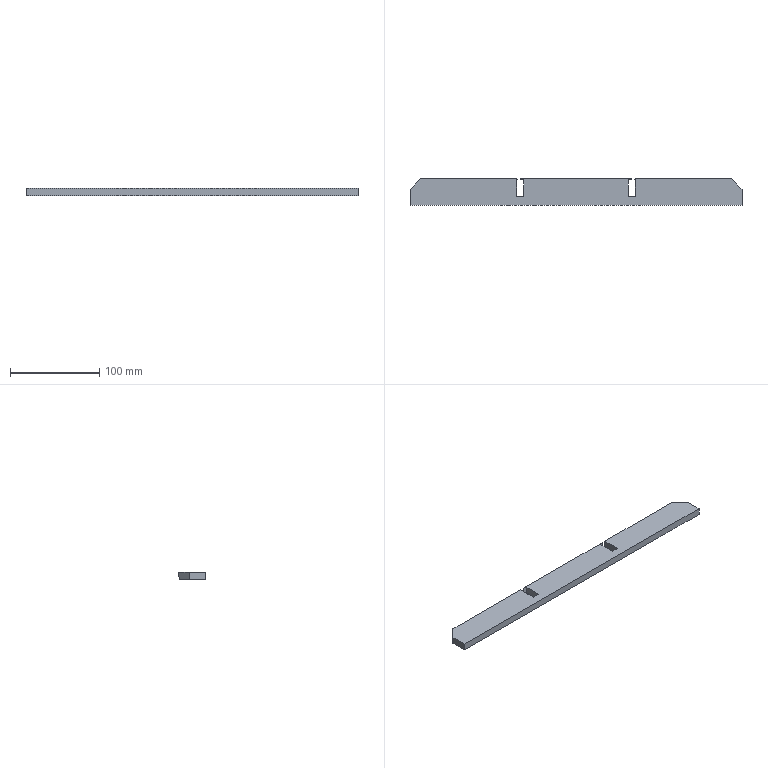Part | SolidWorks | features BaseBody 1 | 1 solid | 18 faces | box 373 x 30 x 8 mm | volume 84961 mm3 | plane 18
STEP:
#1=CARTESIAN_POINT('',(62.311,14.398,0.));
#2=VERTEX_POINT('',#1);
#3=CARTESIAN_POINT('',(62.597,15.,8.));
#4=VERTEX_POINT('',#3);
#5=CARTESIAN_POINT('',(62.311,14.398,0.));
#6=DIRECTION('',(0.0356,0.07493,0.9966));
#7=VECTOR('',#6,1000.);
#8=LINE('',#5,#7);
#9=EDGE_CURVE('',#2,#4,#8,.T.);
#10=ORIENTED_EDGE('',*,*,#9,.F.);
#11=CARTESIAN_POINT('',(-62.311,14.398,0.));
#12=VERTEX_POINT('',#11);
#13=CARTESIAN_POINT('',(0.,14.398,0.));
#14=DIRECTION('',(1.,0.,0.));
#15=VECTOR('',#14,1000.);
#16=LINE('',#13,#15);
#17=EDGE_CURVE('',#12,#2,#16,.T.);
#18=ORIENTED_EDGE('',*,*,#17,.F.);
#19=CARTESIAN_POINT('',(-62.597,15.,8.));
#20=VERTEX_POINT('',#19);
#21=CARTESIAN_POINT('',(-62.597,15.,8.));
#22=DIRECTION('',(0.0356,-0.07493,-0.9966));
#23=VECTOR('',#22,1000.);
#24=LINE('',#21,#23);
#25=EDGE_CURVE('',#20,#12,#24,.T.);
#26=ORIENTED_EDGE('',*,*,#25,.F.);
#27=CARTESIAN_POINT('',(0.,15.,8.));
#28=DIRECTION('',(-1.,0.,0.));
#29=VECTOR('',#28,1000.);
#30=LINE('',#27,#29);
#31=EDGE_CURVE('',#4,#20,#30,.T.);
#32=ORIENTED_EDGE('',*,*,#31,.F.);
#33=EDGE_LOOP('',(#10,#18,#26,#32));
#34=FACE_OUTER_BOUND('',#33,.T.);
#35=CARTESIAN_POINT('',(-63.348,15.,8.));
#36=DIRECTION('',(0.,-0.9972,0.07498));
#37=DIRECTION('',(0.,-0.07498,-0.9972));
#38=AXIS2_PLACEMENT_3D('',#35,#36,#37);
#39=PLANE('',#38);
#40=ADVANCED_FACE('',(#34),#39,.F.);
#41=CARTESIAN_POINT('',(58.61,14.882,8.));
#42=VERTEX_POINT('',#41);
#43=CARTESIAN_POINT('',(62.597,15.,8.));
#44=DIRECTION('',(-0.9996,-0.02956,0.));
#45=VECTOR('',#44,1000.);
#46=LINE('',#43,#45);
#47=EDGE_CURVE('',#4,#42,#46,.T.);
#48=ORIENTED_EDGE('',*,*,#47,.F.);
#49=ORIENTED_EDGE('',*,*,#31,.T.);
#50=CARTESIAN_POINT('',(-58.61,14.882,8.));
#51=VERTEX_POINT('',#50);
#52=CARTESIAN_POINT('',(-58.61,14.882,8.));
#53=DIRECTION('',(-0.9996,0.02956,0.));
#54=VECTOR('',#53,1000.);
#55=LINE('',#52,#54);
#56=EDGE_CURVE('',#51,#20,#55,.T.);
#57=ORIENTED_EDGE('',*,*,#56,.F.);
#58=CARTESIAN_POINT('',(-59.134,-5.166,8.));
#59=VERTEX_POINT('',#58);
#60=CARTESIAN_POINT('',(-59.134,-5.166,8.));
#61=DIRECTION('',(0.02613,0.9997,0.));
#62=VECTOR('',#61,1000.);
#63=LINE('',#60,#62);
#64=EDGE_CURVE('',#59,#51,#63,.T.);
#65=ORIENTED_EDGE('',*,*,#64,.F.);
#66=CARTESIAN_POINT('',(-67.139,-4.929,8.));
#67=VERTEX_POINT('',#66);
#68=CARTESIAN_POINT('',(-67.139,-4.929,8.));
#69=DIRECTION('',(0.9996,-0.02956,0.));
#70=VECTOR('',#69,1000.);
#71=LINE('',#68,#70);
#72=EDGE_CURVE('',#67,#59,#71,.T.);
#73=ORIENTED_EDGE('',*,*,#72,.F.);
#74=CARTESIAN_POINT('',(-66.618,15.,8.));
#75=VERTEX_POINT('',#74);
#76=CARTESIAN_POINT('',(-66.618,15.,8.));
#77=DIRECTION('',(-0.02613,-0.9997,0.));
#78=VECTOR('',#77,1000.);
#79=LINE('',#76,#78);
#80=EDGE_CURVE('',#75,#67,#79,.T.);
#81=ORIENTED_EDGE('',*,*,#80,.F.);
#82=CARTESIAN_POINT('',(-174.5,15.,8.));
#83=VERTEX_POINT('',#82);
#84=CARTESIAN_POINT('',(0.,15.,8.));
#85=DIRECTION('',(1.,0.,0.));
#86=VECTOR('',#85,1000.);
#87=LINE('',#84,#86);
#88=EDGE_CURVE('',#83,#75,#87,.T.);
#89=ORIENTED_EDGE('',*,*,#88,.F.);
#90=CARTESIAN_POINT('',(-186.5,3.,8.));
#91=VERTEX_POINT('',#90);
#92=CARTESIAN_POINT('',(-186.5,3.,8.));
#93=DIRECTION('',(0.7071,0.7071,0.));
#94=VECTOR('',#93,1000.);
#95=LINE('',#92,#94);
#96=EDGE_CURVE('',#91,#83,#95,.T.);
#97=ORIENTED_EDGE('',*,*,#96,.F.);
#98=CARTESIAN_POINT('',(-186.5,-15.,8.));
#99=VERTEX_POINT('',#98);
#100=CARTESIAN_POINT('',(-186.5,0.,8.));
#101=DIRECTION('',(0.,1.,0.));
#102=VECTOR('',#101,1000.);
#103=LINE('',#100,#102);
#104=EDGE_CURVE('',#99,#91,#103,.T.);
#105=ORIENTED_EDGE('',*,*,#104,.F.);
#106=CARTESIAN_POINT('',(186.5,-15.,8.));
#107=VERTEX_POINT('',#106);
#108=CARTESIAN_POINT('',(0.,-15.,8.));
#109=DIRECTION('',(-1.,0.,0.));
#110=VECTOR('',#109,1000.);
#111=LINE('',#108,#110);
#112=EDGE_CURVE('',#107,#99,#111,.T.);
#113=ORIENTED_EDGE('',*,*,#112,.F.);
#114=CARTESIAN_POINT('',(186.5,3.,8.));
#115=VERTEX_POINT('',#114);
#116=CARTESIAN_POINT('',(186.5,0.,8.));
#117=DIRECTION('',(0.,-1.,0.));
#118=VECTOR('',#117,1000.);
#119=LINE('',#116,#118);
#120=EDGE_CURVE('',#115,#107,#119,.T.);
#121=ORIENTED_EDGE('',*,*,#120,.F.);
#122=CARTESIAN_POINT('',(174.5,15.,8.));
#123=VERTEX_POINT('',#122);
#124=CARTESIAN_POINT('',(174.428,15.072,8.));
#125=DIRECTION('',(0.7071,-0.7071,0.));
#126=VECTOR('',#125,1000.);
#127=LINE('',#124,#126);
#128=EDGE_CURVE('',#123,#115,#127,.T.);
#129=ORIENTED_EDGE('',*,*,#128,.F.);
#130=CARTESIAN_POINT('',(66.618,15.,8.));
#131=VERTEX_POINT('',#130);
#132=CARTESIAN_POINT('',(0.,15.,8.));
#133=DIRECTION('',(1.,0.,0.));
#134=VECTOR('',#133,1000.);
#135=LINE('',#132,#134);
#136=EDGE_CURVE('',#131,#123,#135,.T.);
#137=ORIENTED_EDGE('',*,*,#136,.F.);
#138=CARTESIAN_POINT('',(67.139,-4.929,8.));
#139=VERTEX_POINT('',#138);
#140=CARTESIAN_POINT('',(67.139,-4.929,8.));
#141=DIRECTION('',(-0.02613,0.9997,0.));
#142=VECTOR('',#141,1000.);
#143=LINE('',#140,#142);
#144=EDGE_CURVE('',#139,#131,#143,.T.);
#145=ORIENTED_EDGE('',*,*,#144,.F.);
#146=CARTESIAN_POINT('',(59.134,-5.166,8.));
#147=VERTEX_POINT('',#146);
#148=CARTESIAN_POINT('',(59.134,-5.166,8.));
#149=DIRECTION('',(0.9996,0.02956,0.));
#150=VECTOR('',#149,1000.);
#151=LINE('',#148,#150);
#152=EDGE_CURVE('',#147,#139,#151,.T.);
#153=ORIENTED_EDGE('',*,*,#152,.F.);
#154=CARTESIAN_POINT('',(58.61,14.882,8.));
#155=DIRECTION('',(0.02613,-0.9997,0.));
#156=VECTOR('',#155,1000.);
#157=LINE('',#154,#156);
#158=EDGE_CURVE('',#42,#147,#157,.T.);
#159=ORIENTED_EDGE('',*,*,#158,.F.);
#160=EDGE_LOOP('',(#48,#49,#57,#65,#73,#81,#89,#97,#105,#113,#121,#129,#137,#145,#153,#159));
#161=FACE_OUTER_BOUND('',#160,.T.);
#162=CARTESIAN_POINT('',(186.5,-15.,8.));
#163=DIRECTION('',(0.,0.,-1.));
#164=DIRECTION('',(-1.,0.,0.));
#165=AXIS2_PLACEMENT_3D('',#162,#163,#164);
#166=PLANE('',#165);
#167=ADVANCED_FACE('',(#161),#166,.F.);
#168=CARTESIAN_POINT('',(58.255,14.279,0.));
#169=VERTEX_POINT('',#168);
#170=CARTESIAN_POINT('',(62.311,14.398,0.));
#171=DIRECTION('',(-0.9996,-0.02956,0.));
#172=VECTOR('',#171,1000.);
#173=LINE('',#170,#172);
#174=EDGE_CURVE('',#2,#169,#173,.T.);
#175=ORIENTED_EDGE('',*,*,#174,.F.);
#176=ORIENTED_EDGE('',*,*,#9,.T.);
#177=ORIENTED_EDGE('',*,*,#47,.T.);
#178=CARTESIAN_POINT('',(58.255,14.279,0.000000002));
#179=DIRECTION('',(0.04418,0.07516,0.9962));
#180=VECTOR('',#179,1000.);
#181=LINE('',#178,#180);
#182=EDGE_CURVE('',#169,#42,#181,.T.);
#183=ORIENTED_EDGE('',*,*,#182,.F.);
#184=EDGE_LOOP('',(#175,#176,#177,#183));
#185=FACE_OUTER_BOUND('',#184,.T.);
#186=CARTESIAN_POINT('',(58.229,14.274,-0.048));
#187=DIRECTION('',(-0.02948,0.9968,-0.0739));
#188=DIRECTION('',(0.,0.07393,0.9973));
#189=AXIS2_PLACEMENT_3D('',#186,#187,#188);
#190=PLANE('',#189);
#191=ADVANCED_FACE('',(#185),#190,.F.);
#192=CARTESIAN_POINT('',(-58.255,14.279,0.));
#193=VERTEX_POINT('',#192);
#194=CARTESIAN_POINT('',(-58.255,14.279,0.));
#195=DIRECTION('',(-0.9996,0.02956,0.));
#196=VECTOR('',#195,1000.);
#197=LINE('',#194,#196);
#198=EDGE_CURVE('',#193,#12,#197,.T.);
#199=ORIENTED_EDGE('',*,*,#198,.T.);
#200=ORIENTED_EDGE('',*,*,#17,.T.);
#201=ORIENTED_EDGE('',*,*,#174,.T.);
#202=CARTESIAN_POINT('',(58.779,-5.77,0.));
#203=VERTEX_POINT('',#202);
#204=CARTESIAN_POINT('',(58.255,14.279,0.));
#205=DIRECTION('',(0.02613,-0.9997,0.));
#206=VECTOR('',#205,1000.);
#207=LINE('',#204,#206);
#208=EDGE_CURVE('',#169,#203,#207,.T.);
#209=ORIENTED_EDGE('',*,*,#208,.T.);
#210=CARTESIAN_POINT('',(66.784,-5.533,0.));
#211=VERTEX_POINT('',#210);
#212=CARTESIAN_POINT('',(58.779,-5.77,0.));
#213=DIRECTION('',(0.9996,0.02956,0.));
#214=VECTOR('',#213,1000.);
#215=LINE('',#212,#214);
#216=EDGE_CURVE('',#203,#211,#215,.T.);
#217=ORIENTED_EDGE('',*,*,#216,.T.);
#218=CARTESIAN_POINT('',(66.263,14.398,0.));
#219=VERTEX_POINT('',#218);
#220=CARTESIAN_POINT('',(66.784,-5.533,0.));
#221=DIRECTION('',(-0.02613,0.9997,0.));
#222=VECTOR('',#221,1000.);
#223=LINE('',#220,#222);
#224=EDGE_CURVE('',#211,#219,#223,.T.);
#225=ORIENTED_EDGE('',*,*,#224,.T.);
#226=CARTESIAN_POINT('',(175.102,14.398,0.));
#227=VERTEX_POINT('',#226);
#228=CARTESIAN_POINT('',(0.,14.398,0.));
#229=DIRECTION('',(1.,0.,0.));
#230=VECTOR('',#229,1000.);
#231=LINE('',#228,#230);
#232=EDGE_CURVE('',#219,#227,#231,.T.);
#233=ORIENTED_EDGE('',*,*,#232,.T.);
#234=CARTESIAN_POINT('',(186.5,3.,0.));
#235=VERTEX_POINT('',#234);
#236=CARTESIAN_POINT('',(175.102,14.398,0.));
#237=DIRECTION('',(0.7071,-0.7071,0.));
#238=VECTOR('',#237,1000.);
#239=LINE('',#236,#238);
#240=EDGE_CURVE('',#227,#235,#239,.T.);
#241=ORIENTED_EDGE('',*,*,#240,.T.);
#242=CARTESIAN_POINT('',(186.5,-15.,0.));
#243=VERTEX_POINT('',#242);
#244=CARTESIAN_POINT('',(186.5,-0.3008,0.));
#245=DIRECTION('',(0.,-1.,0.));
#246=VECTOR('',#245,1000.);
#247=LINE('',#244,#246);
#248=EDGE_CURVE('',#235,#243,#247,.T.);
#249=ORIENTED_EDGE('',*,*,#248,.T.);
#250=CARTESIAN_POINT('',(-186.5,-15.,0.));
#251=VERTEX_POINT('',#250);
#252=CARTESIAN_POINT('',(0.,-15.,0.));
#253=DIRECTION('',(-1.,0.,0.));
#254=VECTOR('',#253,1000.);
#255=LINE('',#252,#254);
#256=EDGE_CURVE('',#243,#251,#255,.T.);
#257=ORIENTED_EDGE('',*,*,#256,.T.);
#258=CARTESIAN_POINT('',(-186.5,3.,0.));
#259=VERTEX_POINT('',#258);
#260=CARTESIAN_POINT('',(-186.5,-0.3008,0.));
#261=DIRECTION('',(0.,1.,0.));
#262=VECTOR('',#261,1000.);
#263=LINE('',#260,#262);
#264=EDGE_CURVE('',#251,#259,#263,.T.);
#265=ORIENTED_EDGE('',*,*,#264,.T.);
#266=CARTESIAN_POINT('',(-175.102,14.398,0.));
#267=VERTEX_POINT('',#266);
#268=CARTESIAN_POINT('',(-186.5,3.,0.));
#269=DIRECTION('',(0.7071,0.7071,0.));
#270=VECTOR('',#269,1000.);
#271=LINE('',#268,#270);
#272=EDGE_CURVE('',#259,#267,#271,.T.);
#273=ORIENTED_EDGE('',*,*,#272,.T.);
#274=CARTESIAN_POINT('',(-66.263,14.398,0.));
#275=VERTEX_POINT('',#274);
#276=CARTESIAN_POINT('',(0.,14.398,0.));
#277=DIRECTION('',(1.,0.,0.));
#278=VECTOR('',#277,1000.);
#279=LINE('',#276,#278);
#280=EDGE_CURVE('',#267,#275,#279,.T.);
#281=ORIENTED_EDGE('',*,*,#280,.T.);
#282=CARTESIAN_POINT('',(-66.784,-5.533,0.));
#283=VERTEX_POINT('',#282);
#284=CARTESIAN_POINT('',(-66.263,14.398,0.));
#285=DIRECTION('',(-0.02613,-0.9997,0.));
#286=VECTOR('',#285,1000.);
#287=LINE('',#284,#286);
#288=EDGE_CURVE('',#275,#283,#287,.T.);
#289=ORIENTED_EDGE('',*,*,#288,.T.);
#290=CARTESIAN_POINT('',(-58.779,-5.77,0.));
#291=VERTEX_POINT('',#290);
#292=CARTESIAN_POINT('',(-66.784,-5.533,0.));
#293=DIRECTION('',(0.9996,-0.02956,0.));
#294=VECTOR('',#293,1000.);
#295=LINE('',#292,#294);
#296=EDGE_CURVE('',#283,#291,#295,.T.);
#297=ORIENTED_EDGE('',*,*,#296,.T.);
#298=CARTESIAN_POINT('',(-58.779,-5.77,0.));
#299=DIRECTION('',(0.02613,0.9997,0.));
#300=VECTOR('',#299,1000.);
#301=LINE('',#298,#300);
#302=EDGE_CURVE('',#291,#193,#301,.T.);
#303=ORIENTED_EDGE('',*,*,#302,.T.);
#304=EDGE_LOOP('',(#199,#200,#201,#209,#217,#225,#233,#241,#249,#257,#265,#273,#281,#289,#297,#303));
#305=FACE_OUTER_BOUND('',#304,.T.);
#306=CARTESIAN_POINT('',(186.5,-15.,0.));
#307=DIRECTION('',(0.,0.,-1.));
#308=DIRECTION('',(-1.,0.,0.));
#309=AXIS2_PLACEMENT_3D('',#306,#307,#308);
#310=PLANE('',#309);
#311=ADVANCED_FACE('',(#305),#310,.T.);
#312=ORIENTED_EDGE('',*,*,#198,.F.);
#313=CARTESIAN_POINT('',(-58.61,14.882,8.));
#314=DIRECTION('',(0.04418,-0.07516,-0.9962));
#315=VECTOR('',#314,1000.);
#316=LINE('',#313,#315);
#317=EDGE_CURVE('',#51,#193,#316,.T.);
#318=ORIENTED_EDGE('',*,*,#317,.F.);
#319=ORIENTED_EDGE('',*,*,#56,.T.);
#320=ORIENTED_EDGE('',*,*,#25,.T.);
#321=EDGE_LOOP('',(#312,#318,#319,#320));
#322=FACE_OUTER_BOUND('',#321,.T.);
#323=CARTESIAN_POINT('',(-62.623,14.403,-0.05758));
#324=DIRECTION('',(0.02948,0.9968,-0.0739));
#325=DIRECTION('',(0.,0.07393,0.9973));
#326=AXIS2_PLACEMENT_3D('',#323,#324,#325);
#327=PLANE('',#326);
#328=ADVANCED_FACE('',(#322),#327,.F.);
#329=ORIENTED_EDGE('',*,*,#208,.F.);
#330=ORIENTED_EDGE('',*,*,#182,.T.);
#331=ORIENTED_EDGE('',*,*,#158,.T.);
#332=CARTESIAN_POINT('',(58.779,-5.77,0.000000003));
#333=DIRECTION('',(0.04418,0.07516,0.9962));
#334=VECTOR('',#333,1000.);
#335=LINE('',#332,#334);
#336=EDGE_CURVE('',#203,#147,#335,.T.);
#337=ORIENTED_EDGE('',*,*,#336,.F.);
#338=EDGE_LOOP('',(#329,#330,#331,#337));
#339=FACE_OUTER_BOUND('',#338,.T.);
#340=CARTESIAN_POINT('',(58.779,-5.893,-0.07251));
#341=DIRECTION('',(-0.9986,-0.0261,0.04626));
#342=DIRECTION('',(0.04627,0.,0.9989));
#343=AXIS2_PLACEMENT_3D('',#340,#341,#342);
#344=PLANE('',#343);
#345=ADVANCED_FACE('',(#339),#344,.F.);
#346=ORIENTED_EDGE('',*,*,#302,.F.);
#347=CARTESIAN_POINT('',(-59.134,-5.166,8.));
#348=DIRECTION('',(0.04418,-0.07516,-0.9962));
#349=VECTOR('',#348,1000.);
#350=LINE('',#347,#349);
#351=EDGE_CURVE('',#59,#291,#350,.T.);
#352=ORIENTED_EDGE('',*,*,#351,.F.);
#353=ORIENTED_EDGE('',*,*,#64,.T.);
#354=ORIENTED_EDGE('',*,*,#317,.T.);
#355=EDGE_LOOP('',(#346,#352,#353,#354));
#356=FACE_OUTER_BOUND('',#355,.T.);
#357=CARTESIAN_POINT('',(-59.155,-5.893,8.047));
#358=DIRECTION('',(0.9986,-0.0261,0.04626));
#359=DIRECTION('',(0.04627,0.,-0.9989));
#360=AXIS2_PLACEMENT_3D('',#357,#358,#359);
#361=PLANE('',#360);
#362=ADVANCED_FACE('',(#356),#361,.F.);
#363=ORIENTED_EDGE('',*,*,#296,.F.);
#364=CARTESIAN_POINT('',(-67.139,-4.929,8.));
#365=DIRECTION('',(0.04418,-0.07516,-0.9962));
#366=VECTOR('',#365,1000.);
#367=LINE('',#364,#366);
#368=EDGE_CURVE('',#67,#283,#367,.T.);
#369=ORIENTED_EDGE('',*,*,#368,.F.);
#370=ORIENTED_EDGE('',*,*,#72,.T.);
#371=ORIENTED_EDGE('',*,*,#351,.T.);
#372=EDGE_LOOP('',(#363,#369,#370,#371));
#373=FACE_OUTER_BOUND('',#372,.T.);
#374=CARTESIAN_POINT('',(-67.189,-4.924,8.048));
#375=DIRECTION('',(-0.02948,-0.9968,0.0739));
#376=DIRECTION('',(0.,-0.07393,-0.9973));
#377=AXIS2_PLACEMENT_3D('',#374,#375,#376);
#378=PLANE('',#377);
#379=ADVANCED_FACE('',(#373),#378,.F.);
#380=ORIENTED_EDGE('',*,*,#288,.F.);
#381=CARTESIAN_POINT('',(-66.618,15.,8.));
#382=DIRECTION('',(0.04419,-0.07491,-0.9962));
#383=VECTOR('',#382,1000.);
#384=LINE('',#381,#383);
#385=EDGE_CURVE('',#75,#275,#384,.T.);
#386=ORIENTED_EDGE('',*,*,#385,.F.);
#387=ORIENTED_EDGE('',*,*,#80,.T.);
#388=ORIENTED_EDGE('',*,*,#368,.T.);
#389=EDGE_LOOP('',(#380,#386,#387,#388));
#390=FACE_OUTER_BOUND('',#389,.T.);
#391=CARTESIAN_POINT('',(-66.784,-5.656,-0.07237));
#392=DIRECTION('',(-0.9986,0.0261,-0.04626));
#393=DIRECTION('',(-0.04627,0.,0.9989));
#394=AXIS2_PLACEMENT_3D('',#391,#392,#393);
#395=PLANE('',#394);
#396=ADVANCED_FACE('',(#390),#395,.F.);
#397=ORIENTED_EDGE('',*,*,#385,.T.);
#398=ORIENTED_EDGE('',*,*,#280,.F.);
#399=CARTESIAN_POINT('',(-174.5,15.,8.));
#400=DIRECTION('',(-0.07477,-0.07477,-0.9944));
#401=VECTOR('',#400,1000.);
#402=LINE('',#399,#401);
#403=EDGE_CURVE('',#83,#267,#402,.T.);
#404=ORIENTED_EDGE('',*,*,#403,.F.);
#405=ORIENTED_EDGE('',*,*,#88,.T.);
#406=EDGE_LOOP('',(#397,#398,#404,#405));
#407=FACE_OUTER_BOUND('',#406,.T.);
#408=CARTESIAN_POINT('',(-175.755,15.,8.));
#409=DIRECTION('',(0.,-0.9972,0.07498));
#410=DIRECTION('',(0.,-0.07498,-0.9972));
#411=AXIS2_PLACEMENT_3D('',#408,#409,#410);
#412=PLANE('',#411);
#413=ADVANCED_FACE('',(#407),#412,.F.);
#414=ORIENTED_EDGE('',*,*,#403,.T.);
#415=ORIENTED_EDGE('',*,*,#272,.F.);
#416=CARTESIAN_POINT('',(-186.5,3.,4.));
#417=DIRECTION('',(0.,0.,-1.));
#418=VECTOR('',#417,1000.);
#419=LINE('',#416,#418);
#420=EDGE_CURVE('',#91,#259,#419,.T.);
#421=ORIENTED_EDGE('',*,*,#420,.F.);
#422=ORIENTED_EDGE('',*,*,#96,.T.);
#423=EDGE_LOOP('',(#414,#415,#421,#422));
#424=FACE_OUTER_BOUND('',#423,.T.);
#425=CARTESIAN_POINT('',(-186.5,3.,0.));
#426=DIRECTION('',(0.7071,-0.7071,0.));
#427=DIRECTION('',(0.7071,0.7071,0.));
#428=AXIS2_PLACEMENT_3D('',#425,#426,#427);
#429=PLANE('',#428);
#430=ADVANCED_FACE('',(#424),#429,.F.);
#431=CARTESIAN_POINT('',(-186.5,-15.,4.));
#432=DIRECTION('',(0.,0.,-1.));
#433=VECTOR('',#432,1000.);
#434=LINE('',#431,#433);
#435=EDGE_CURVE('',#99,#251,#434,.T.);
#436=ORIENTED_EDGE('',*,*,#435,.F.);
#437=ORIENTED_EDGE('',*,*,#104,.T.);
#438=ORIENTED_EDGE('',*,*,#420,.T.);
#439=ORIENTED_EDGE('',*,*,#264,.F.);
#440=EDGE_LOOP('',(#436,#437,#438,#439));
#441=FACE_OUTER_BOUND('',#440,.T.);
#442=CARTESIAN_POINT('',(-186.5,-15.,8.));
#443=DIRECTION('',(1.,0.,0.));
#444=DIRECTION('',(0.,0.,-1.));
#445=AXIS2_PLACEMENT_3D('',#442,#443,#444);
#446=PLANE('',#445);
#447=ADVANCED_FACE('',(#441),#446,.F.);
#448=CARTESIAN_POINT('',(186.5,-15.,4.));
#449=DIRECTION('',(0.,0.,-1.));
#450=VECTOR('',#449,1000.);
#451=LINE('',#448,#450);
#452=EDGE_CURVE('',#107,#243,#451,.T.);
#453=ORIENTED_EDGE('',*,*,#452,.F.);
#454=ORIENTED_EDGE('',*,*,#112,.T.);
#455=ORIENTED_EDGE('',*,*,#435,.T.);
#456=ORIENTED_EDGE('',*,*,#256,.F.);
#457=EDGE_LOOP('',(#453,#454,#455,#456));
#458=FACE_OUTER_BOUND('',#457,.T.);
#459=CARTESIAN_POINT('',(186.5,-15.,0.));
#460=DIRECTION('',(0.,1.,0.));
#461=DIRECTION('',(-1.,0.,0.));
#462=AXIS2_PLACEMENT_3D('',#459,#460,#461);
#463=PLANE('',#462);
#464=ADVANCED_FACE('',(#458),#463,.F.);
#465=CARTESIAN_POINT('',(186.5,3.,4.));
#466=DIRECTION('',(0.,0.,-1.));
#467=VECTOR('',#466,1000.);
#468=LINE('',#465,#467);
#469=EDGE_CURVE('',#115,#235,#468,.T.);
#470=ORIENTED_EDGE('',*,*,#469,.F.);
#471=ORIENTED_EDGE('',*,*,#120,.T.);
#472=ORIENTED_EDGE('',*,*,#452,.T.);
#473=ORIENTED_EDGE('',*,*,#248,.F.);
#474=EDGE_LOOP('',(#470,#471,#472,#473));
#475=FACE_OUTER_BOUND('',#474,.T.);
#476=CARTESIAN_POINT('',(186.5,-15.,0.));
#477=DIRECTION('',(-1.,0.,0.));
#478=DIRECTION('',(0.,0.,1.));
#479=AXIS2_PLACEMENT_3D('',#476,#477,#478);
#480=PLANE('',#479);
#481=ADVANCED_FACE('',(#475),#480,.F.);
#482=CARTESIAN_POINT('',(174.5,15.,8.));
#483=DIRECTION('',(0.07477,-0.07477,-0.9944));
#484=VECTOR('',#483,1000.);
#485=LINE('',#482,#484);
#486=EDGE_CURVE('',#123,#227,#485,.T.);
#487=ORIENTED_EDGE('',*,*,#486,.F.);
#488=ORIENTED_EDGE('',*,*,#128,.T.);
#489=ORIENTED_EDGE('',*,*,#469,.T.);
#490=ORIENTED_EDGE('',*,*,#240,.F.);
#491=EDGE_LOOP('',(#487,#488,#489,#490));
#492=FACE_OUTER_BOUND('',#491,.T.);
#493=CARTESIAN_POINT('',(174.428,15.072,0.));
#494=DIRECTION('',(-0.7071,-0.7071,0.));
#495=DIRECTION('',(0.7071,-0.7071,0.));
#496=AXIS2_PLACEMENT_3D('',#493,#494,#495);
#497=PLANE('',#496);
#498=ADVANCED_FACE('',(#492),#497,.F.);
#499=CARTESIAN_POINT('',(66.618,15.,8.));
#500=DIRECTION('',(-0.04419,-0.07491,-0.9962));
#501=VECTOR('',#500,1000.);
#502=LINE('',#499,#501);
#503=EDGE_CURVE('',#131,#219,#502,.T.);
#504=ORIENTED_EDGE('',*,*,#503,.F.);
#505=ORIENTED_EDGE('',*,*,#136,.T.);
#506=ORIENTED_EDGE('',*,*,#486,.T.);
#507=ORIENTED_EDGE('',*,*,#232,.F.);
#508=EDGE_LOOP('',(#504,#505,#506,#507));
#509=FACE_OUTER_BOUND('',#508,.T.);
#510=CARTESIAN_POINT('',(65.61,15.,8.));
#511=DIRECTION('',(0.,-0.9972,0.07498));
#512=DIRECTION('',(0.,-0.07498,-0.9972));
#513=AXIS2_PLACEMENT_3D('',#510,#511,#512);
#514=PLANE('',#513);
#515=ADVANCED_FACE('',(#509),#514,.F.);
#516=ORIENTED_EDGE('',*,*,#224,.F.);
#517=CARTESIAN_POINT('',(67.139,-4.929,8.));
#518=DIRECTION('',(-0.04418,-0.07516,-0.9962));
#519=VECTOR('',#518,1000.);
#520=LINE('',#517,#519);
#521=EDGE_CURVE('',#139,#211,#520,.T.);
#522=ORIENTED_EDGE('',*,*,#521,.F.);
#523=ORIENTED_EDGE('',*,*,#144,.T.);
#524=ORIENTED_EDGE('',*,*,#503,.T.);
#525=EDGE_LOOP('',(#516,#522,#523,#524));
#526=FACE_OUTER_BOUND('',#525,.T.);
#527=CARTESIAN_POINT('',(67.16,-5.656,8.047));
#528=DIRECTION('',(0.9986,0.0261,-0.04626));
#529=DIRECTION('',(-0.04627,0.,-0.9989));
#530=AXIS2_PLACEMENT_3D('',#527,#528,#529);
#531=PLANE('',#530);
#532=ADVANCED_FACE('',(#526),#531,.F.);
#533=ORIENTED_EDGE('',*,*,#216,.F.);
#534=ORIENTED_EDGE('',*,*,#336,.T.);
#535=ORIENTED_EDGE('',*,*,#152,.T.);
#536=ORIENTED_EDGE('',*,*,#521,.T.);
#537=EDGE_LOOP('',(#533,#534,#535,#536));
#538=FACE_OUTER_BOUND('',#537,.T.);
#539=CARTESIAN_POINT('',(58.729,-5.173,8.066));
#540=DIRECTION('',(0.02948,-0.9968,0.0739));
#541=DIRECTION('',(0.,-0.07393,-0.9973));
#542=AXIS2_PLACEMENT_3D('',#539,#540,#541);
#543=PLANE('',#542);
#544=ADVANCED_FACE('',(#538),#543,.F.);
#545=CLOSED_SHELL('',(#40,#167,#191,#311,#328,#345,#362,#379,#396,#413,#430,#447,#464,#481,#498,#515,#532,#544));
#546=MANIFOLD_SOLID_BREP('',#545);
#547=CARTESIAN_POINT('',(0.,0.,0.));
#548=DIRECTION('',(0.,0.,1.));
#549=DIRECTION('',(1.,0.,0.));
#550=AXIS2_PLACEMENT_3D('',#547,#548,#549);
#551=(LENGTH_UNIT()NAMED_UNIT(*)SI_UNIT(.MILLI.,.METRE.));
#552=UNCERTAINTY_MEASURE_WITH_UNIT(LENGTH_MEASURE(0.00001),#551,'','');
#553=(NAMED_UNIT(*)PLANE_ANGLE_UNIT()SI_UNIT($,.RADIAN.));
#554=(NAMED_UNIT(*)SI_UNIT($,.STERADIAN.)SOLID_ANGLE_UNIT());
#555=(GEOMETRIC_REPRESENTATION_CONTEXT(3)GLOBAL_UNCERTAINTY_ASSIGNED_CONTEXT((#552))GLOBAL_UNIT_ASSIGNED_CONTEXT((#551,#553,#554))REPRESENTATION_CONTEXT('',''));
#556=ADVANCED_BREP_SHAPE_REPRESENTATION('',(#546,#550),#555);